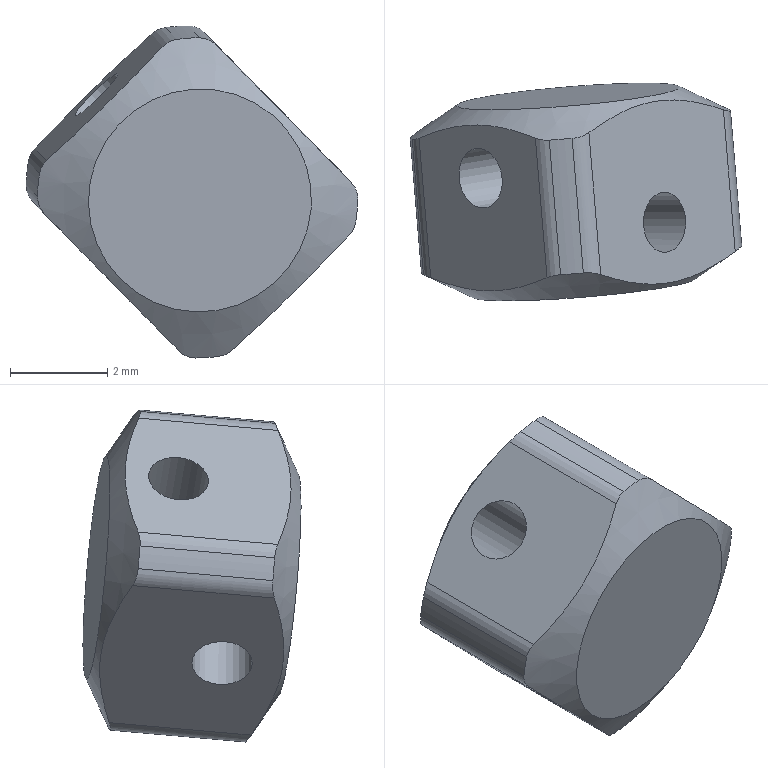Part | STEP file | Wytnij-wyci_gni_cie2_4 | 1 solid | 22 faces | box 6.818 x 4.485 x 6.828 mm | volume 88.126 mm3 | cylinder 14 | plane 6 | cone 2 | commonest cylinder face diameters 1 x8 6.61 x4 1.24 x2